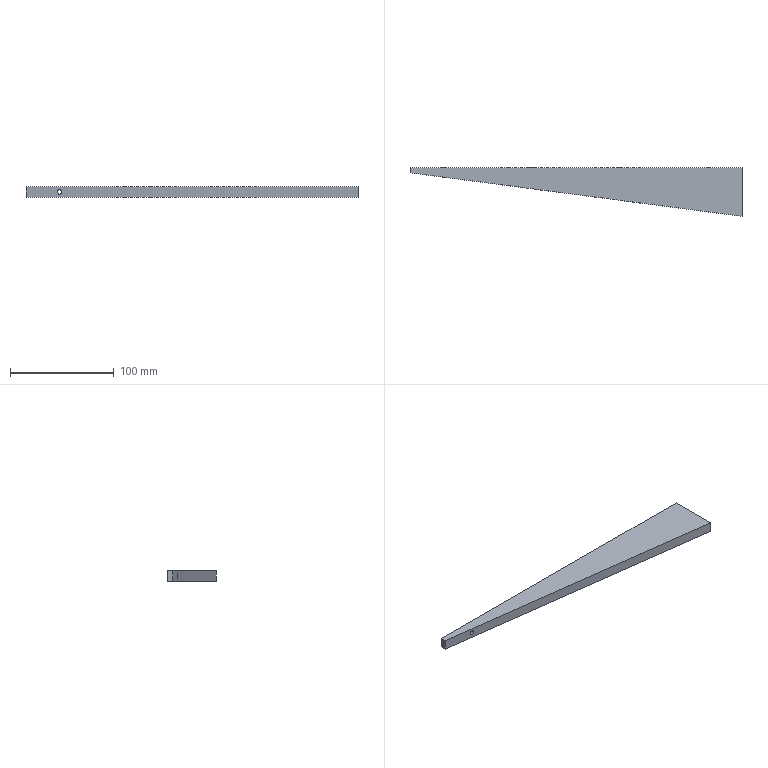Part | SolidWorks | features HoleWzd 2, Extrusion 1 | 1 solid | 32 faces | box 320 x 47 x 10 mm | volume 81873 mm3 | cylinder 14 | cone 12 | plane 6 | commonest cylinder face diameters 4.2 x14
STEP:
#1=CARTESIAN_POINT('',(-14.,41.,7.1));
#2=VERTEX_POINT('',#1);
#3=CARTESIAN_POINT('',(-14.,41.,2.9));
#4=VERTEX_POINT('',#3);
#5=CARTESIAN_POINT('',(-14.,41.,5.));
#6=DIRECTION('',(1.,0.,0.));
#7=DIRECTION('',(0.,0.,-1.));
#8=AXIS2_PLACEMENT_3D('',#5,#6,#7);
#9=CIRCLE('',#8,2.1);
#10=EDGE_CURVE('',#2,#4,#9,.T.);
#11=ORIENTED_EDGE('',*,*,#10,.F.);
#12=CARTESIAN_POINT('',(0.,41.,7.1));
#13=VERTEX_POINT('',#12);
#14=CARTESIAN_POINT('',(0.,41.,7.1));
#15=DIRECTION('',(1.,0.,0.));
#16=VECTOR('',#15,1000.);
#17=LINE('',#14,#16);
#18=EDGE_CURVE('',#2,#13,#17,.T.);
#19=ORIENTED_EDGE('',*,*,#18,.T.);
#20=CARTESIAN_POINT('',(0.,41.,2.9));
#21=VERTEX_POINT('',#20);
#22=CARTESIAN_POINT('',(0.,41.,5.));
#23=DIRECTION('',(1.,0.,0.));
#24=DIRECTION('',(0.,0.,-1.));
#25=AXIS2_PLACEMENT_3D('',#22,#23,#24);
#26=CIRCLE('',#25,2.1);
#27=EDGE_CURVE('',#13,#21,#26,.T.);
#28=ORIENTED_EDGE('',*,*,#27,.T.);
#29=CARTESIAN_POINT('',(0.,41.,2.9));
#30=DIRECTION('',(1.,0.,0.));
#31=VECTOR('',#30,1000.);
#32=LINE('',#29,#31);
#33=EDGE_CURVE('',#4,#21,#32,.T.);
#34=ORIENTED_EDGE('',*,*,#33,.F.);
#35=EDGE_LOOP('',(#11,#19,#28,#34));
#36=FACE_OUTER_BOUND('',#35,.T.);
#37=CARTESIAN_POINT('',(0.,41.,5.));
#38=DIRECTION('',(1.,0.,0.));
#39=DIRECTION('',(0.,0.,-1.));
#40=AXIS2_PLACEMENT_3D('',#37,#38,#39);
#41=CYLINDRICAL_SURFACE('',#40,2.1);
#42=ADVANCED_FACE('',(#36),#41,.F.);
#43=CARTESIAN_POINT('',(-15.262,41.,5.));
#44=VERTEX_POINT('',#43);
#45=CARTESIAN_POINT('',(-14.,41.,2.9));
#46=DIRECTION('',(0.515,0.,-0.8572));
#47=VECTOR('',#46,1000.);
#48=LINE('',#45,#47);
#49=EDGE_CURVE('',#44,#4,#48,.T.);
#50=ORIENTED_EDGE('',*,*,#49,.F.);
#51=CARTESIAN_POINT('',(-14.,41.,7.1));
#52=DIRECTION('',(0.515,0.,0.8572));
#53=VECTOR('',#52,1000.);
#54=LINE('',#51,#53);
#55=EDGE_CURVE('',#44,#2,#54,.T.);
#56=ORIENTED_EDGE('',*,*,#55,.T.);
#57=ORIENTED_EDGE('',*,*,#10,.T.);
#58=EDGE_LOOP('',(#50,#56,#57));
#59=FACE_OUTER_BOUND('',#58,.T.);
#60=CARTESIAN_POINT('',(-14.,41.,5.));
#61=DIRECTION('',(1.,0.,0.));
#62=DIRECTION('',(0.,0.,-1.));
#63=AXIS2_PLACEMENT_3D('',#60,#61,#62);
#64=CONICAL_SURFACE('',#63,2.1,1.03);
#65=ADVANCED_FACE('',(#59),#64,.F.);
#66=CARTESIAN_POINT('',(-14.,25.,7.1));
#67=VERTEX_POINT('',#66);
#68=CARTESIAN_POINT('',(-14.,25.,2.9));
#69=VERTEX_POINT('',#68);
#70=CARTESIAN_POINT('',(-14.,25.,5.));
#71=DIRECTION('',(1.,0.,0.));
#72=DIRECTION('',(0.,0.,-1.));
#73=AXIS2_PLACEMENT_3D('',#70,#71,#72);
#74=CIRCLE('',#73,2.1);
#75=EDGE_CURVE('',#67,#69,#74,.T.);
#76=ORIENTED_EDGE('',*,*,#75,.F.);
#77=CARTESIAN_POINT('',(0.,25.,7.1));
#78=VERTEX_POINT('',#77);
#79=CARTESIAN_POINT('',(0.,25.,7.1));
#80=DIRECTION('',(1.,0.,0.));
#81=VECTOR('',#80,1000.);
#82=LINE('',#79,#81);
#83=EDGE_CURVE('',#67,#78,#82,.T.);
#84=ORIENTED_EDGE('',*,*,#83,.T.);
#85=CARTESIAN_POINT('',(0.,25.,2.9));
#86=VERTEX_POINT('',#85);
#87=CARTESIAN_POINT('',(0.,25.,5.));
#88=DIRECTION('',(1.,0.,0.));
#89=DIRECTION('',(0.,0.,-1.));
#90=AXIS2_PLACEMENT_3D('',#87,#88,#89);
#91=CIRCLE('',#90,2.1);
#92=EDGE_CURVE('',#78,#86,#91,.T.);
#93=ORIENTED_EDGE('',*,*,#92,.T.);
#94=CARTESIAN_POINT('',(0.,25.,2.9));
#95=DIRECTION('',(1.,0.,0.));
#96=VECTOR('',#95,1000.);
#97=LINE('',#94,#96);
#98=EDGE_CURVE('',#69,#86,#97,.T.);
#99=ORIENTED_EDGE('',*,*,#98,.F.);
#100=EDGE_LOOP('',(#76,#84,#93,#99));
#101=FACE_OUTER_BOUND('',#100,.T.);
#102=CARTESIAN_POINT('',(0.,25.,5.));
#103=DIRECTION('',(1.,0.,0.));
#104=DIRECTION('',(0.,0.,-1.));
#105=AXIS2_PLACEMENT_3D('',#102,#103,#104);
#106=CYLINDRICAL_SURFACE('',#105,2.1);
#107=ADVANCED_FACE('',(#101),#106,.F.);
#108=CARTESIAN_POINT('',(-15.262,25.,5.));
#109=VERTEX_POINT('',#108);
#110=CARTESIAN_POINT('',(-14.,25.,2.9));
#111=DIRECTION('',(0.515,0.,-0.8572));
#112=VECTOR('',#111,1000.);
#113=LINE('',#110,#112);
#114=EDGE_CURVE('',#109,#69,#113,.T.);
#115=ORIENTED_EDGE('',*,*,#114,.F.);
#116=CARTESIAN_POINT('',(-14.,25.,7.1));
#117=DIRECTION('',(0.515,0.,0.8572));
#118=VECTOR('',#117,1000.);
#119=LINE('',#116,#118);
#120=EDGE_CURVE('',#109,#67,#119,.T.);
#121=ORIENTED_EDGE('',*,*,#120,.T.);
#122=ORIENTED_EDGE('',*,*,#75,.T.);
#123=EDGE_LOOP('',(#115,#121,#122));
#124=FACE_OUTER_BOUND('',#123,.T.);
#125=CARTESIAN_POINT('',(-14.,25.,5.));
#126=DIRECTION('',(1.,0.,0.));
#127=DIRECTION('',(0.,0.,-1.));
#128=AXIS2_PLACEMENT_3D('',#125,#126,#127);
#129=CONICAL_SURFACE('',#128,2.1,1.03);
#130=ADVANCED_FACE('',(#124),#129,.F.);
#131=CARTESIAN_POINT('',(-14.,9.,7.1));
#132=VERTEX_POINT('',#131);
#133=CARTESIAN_POINT('',(-14.,9.,2.9));
#134=VERTEX_POINT('',#133);
#135=CARTESIAN_POINT('',(-14.,9.,5.));
#136=DIRECTION('',(1.,0.,0.));
#137=DIRECTION('',(0.,0.,-1.));
#138=AXIS2_PLACEMENT_3D('',#135,#136,#137);
#139=CIRCLE('',#138,2.1);
#140=EDGE_CURVE('',#132,#134,#139,.T.);
#141=ORIENTED_EDGE('',*,*,#140,.F.);
#142=CARTESIAN_POINT('',(0.,9.,7.1));
#143=VERTEX_POINT('',#142);
#144=CARTESIAN_POINT('',(0.,9.,7.1));
#145=DIRECTION('',(1.,0.,0.));
#146=VECTOR('',#145,1000.);
#147=LINE('',#144,#146);
#148=EDGE_CURVE('',#132,#143,#147,.T.);
#149=ORIENTED_EDGE('',*,*,#148,.T.);
#150=CARTESIAN_POINT('',(0.,9.,2.9));
#151=VERTEX_POINT('',#150);
#152=CARTESIAN_POINT('',(0.,9.,5.));
#153=DIRECTION('',(1.,0.,0.));
#154=DIRECTION('',(0.,0.,-1.));
#155=AXIS2_PLACEMENT_3D('',#152,#153,#154);
#156=CIRCLE('',#155,2.1);
#157=EDGE_CURVE('',#143,#151,#156,.T.);
#158=ORIENTED_EDGE('',*,*,#157,.T.);
#159=CARTESIAN_POINT('',(0.,9.,2.9));
#160=DIRECTION('',(1.,0.,0.));
#161=VECTOR('',#160,1000.);
#162=LINE('',#159,#161);
#163=EDGE_CURVE('',#134,#151,#162,.T.);
#164=ORIENTED_EDGE('',*,*,#163,.F.);
#165=EDGE_LOOP('',(#141,#149,#158,#164));
#166=FACE_OUTER_BOUND('',#165,.T.);
#167=CARTESIAN_POINT('',(0.,9.,5.));
#168=DIRECTION('',(1.,0.,0.));
#169=DIRECTION('',(0.,0.,-1.));
#170=AXIS2_PLACEMENT_3D('',#167,#168,#169);
#171=CYLINDRICAL_SURFACE('',#170,2.1);
#172=ADVANCED_FACE('',(#166),#171,.F.);
#173=CARTESIAN_POINT('',(-15.262,9.,5.));
#174=VERTEX_POINT('',#173);
#175=CARTESIAN_POINT('',(-14.,9.,2.9));
#176=DIRECTION('',(0.515,0.,-0.8572));
#177=VECTOR('',#176,1000.);
#178=LINE('',#175,#177);
#179=EDGE_CURVE('',#174,#134,#178,.T.);
#180=ORIENTED_EDGE('',*,*,#179,.F.);
#181=CARTESIAN_POINT('',(-14.,9.,7.1));
#182=DIRECTION('',(0.515,0.,0.8572));
#183=VECTOR('',#182,1000.);
#184=LINE('',#181,#183);
#185=EDGE_CURVE('',#174,#132,#184,.T.);
#186=ORIENTED_EDGE('',*,*,#185,.T.);
#187=ORIENTED_EDGE('',*,*,#140,.T.);
#188=EDGE_LOOP('',(#180,#186,#187));
#189=FACE_OUTER_BOUND('',#188,.T.);
#190=CARTESIAN_POINT('',(-14.,9.,5.));
#191=DIRECTION('',(1.,0.,0.));
#192=DIRECTION('',(0.,0.,-1.));
#193=AXIS2_PLACEMENT_3D('',#190,#191,#192);
#194=CONICAL_SURFACE('',#193,2.1,1.03);
#195=ADVANCED_FACE('',(#189),#194,.F.);
#196=CARTESIAN_POINT('',(-287.5,37.734,2.9));
#197=VERTEX_POINT('',#196);
#198=CARTESIAN_POINT('',(-287.5,37.734,7.1));
#199=VERTEX_POINT('',#198);
#200=CARTESIAN_POINT('',(-287.5,37.734,2.9));
#201=CARTESIAN_POINT('',(-291.7,38.286,2.9));
#202=CARTESIAN_POINT('',(-291.7,38.286,7.1));
#203=CARTESIAN_POINT('',(-287.5,37.734,7.1));
#204=(BOUNDED_CURVE()B_SPLINE_CURVE(3,(#200,#201,#202,#203),.UNSPECIFIED.,.F.,.F.)B_SPLINE_CURVE_WITH_KNOTS((4,4),(4.712,7.854),.UNSPECIFIED.)CURVE()GEOMETRIC_REPRESENTATION_ITEM()RATIONAL_B_SPLINE_CURVE((1.,0.3333,0.3333,1.))REPRESENTATION_ITEM(''));
#205=EDGE_CURVE('',#197,#199,#204,.T.);
#206=ORIENTED_EDGE('',*,*,#205,.F.);
#207=CARTESIAN_POINT('',(-287.5,47.,2.9));
#208=VERTEX_POINT('',#207);
#209=CARTESIAN_POINT('',(-287.5,47.,2.9));
#210=DIRECTION('',(0.,1.,0.));
#211=VECTOR('',#210,1000.);
#212=LINE('',#209,#211);
#213=EDGE_CURVE('',#197,#208,#212,.T.);
#214=ORIENTED_EDGE('',*,*,#213,.T.);
#215=CARTESIAN_POINT('',(-287.5,47.,7.1));
#216=VERTEX_POINT('',#215);
#217=CARTESIAN_POINT('',(-287.5,47.,5.));
#218=DIRECTION('',(0.,1.,0.));
#219=DIRECTION('',(0.,0.,1.));
#220=AXIS2_PLACEMENT_3D('',#217,#218,#219);
#221=CIRCLE('',#220,2.1);
#222=EDGE_CURVE('',#208,#216,#221,.T.);
#223=ORIENTED_EDGE('',*,*,#222,.T.);
#224=CARTESIAN_POINT('',(-287.5,47.,7.1));
#225=DIRECTION('',(0.,1.,0.));
#226=VECTOR('',#225,1000.);
#227=LINE('',#224,#226);
#228=EDGE_CURVE('',#199,#216,#227,.T.);
#229=ORIENTED_EDGE('',*,*,#228,.F.);
#230=EDGE_LOOP('',(#206,#214,#223,#229));
#231=FACE_OUTER_BOUND('',#230,.T.);
#232=CARTESIAN_POINT('',(-287.5,47.,5.));
#233=DIRECTION('',(0.,1.,0.));
#234=DIRECTION('',(0.,0.,1.));
#235=AXIS2_PLACEMENT_3D('',#232,#233,#234);
#236=CYLINDRICAL_SURFACE('',#235,2.1);
#237=ADVANCED_FACE('',(#231),#236,.F.);
#238=CARTESIAN_POINT('',(-202.5,33.,2.9));
#239=VERTEX_POINT('',#238);
#240=CARTESIAN_POINT('',(-202.5,33.,7.1));
#241=VERTEX_POINT('',#240);
#242=CARTESIAN_POINT('',(-202.5,33.,5.));
#243=DIRECTION('',(0.,1.,0.));
#244=DIRECTION('',(0.,0.,1.));
#245=AXIS2_PLACEMENT_3D('',#242,#243,#244);
#246=CIRCLE('',#245,2.1);
#247=EDGE_CURVE('',#239,#241,#246,.T.);
#248=ORIENTED_EDGE('',*,*,#247,.F.);
#249=CARTESIAN_POINT('',(-202.5,47.,2.9));
#250=VERTEX_POINT('',#249);
#251=CARTESIAN_POINT('',(-202.5,47.,2.9));
#252=DIRECTION('',(0.,1.,0.));
#253=VECTOR('',#252,1000.);
#254=LINE('',#251,#253);
#255=EDGE_CURVE('',#239,#250,#254,.T.);
#256=ORIENTED_EDGE('',*,*,#255,.T.);
#257=CARTESIAN_POINT('',(-202.5,47.,7.1));
#258=VERTEX_POINT('',#257);
#259=CARTESIAN_POINT('',(-202.5,47.,5.));
#260=DIRECTION('',(0.,1.,0.));
#261=DIRECTION('',(0.,0.,1.));
#262=AXIS2_PLACEMENT_3D('',#259,#260,#261);
#263=CIRCLE('',#262,2.1);
#264=EDGE_CURVE('',#250,#258,#263,.T.);
#265=ORIENTED_EDGE('',*,*,#264,.T.);
#266=CARTESIAN_POINT('',(-202.5,47.,7.1));
#267=DIRECTION('',(0.,1.,0.));
#268=VECTOR('',#267,1000.);
#269=LINE('',#266,#268);
#270=EDGE_CURVE('',#241,#258,#269,.T.);
#271=ORIENTED_EDGE('',*,*,#270,.F.);
#272=EDGE_LOOP('',(#248,#256,#265,#271));
#273=FACE_OUTER_BOUND('',#272,.T.);
#274=CARTESIAN_POINT('',(-202.5,47.,5.));
#275=DIRECTION('',(0.,1.,0.));
#276=DIRECTION('',(0.,0.,1.));
#277=AXIS2_PLACEMENT_3D('',#274,#275,#276);
#278=CYLINDRICAL_SURFACE('',#277,2.1);
#279=ADVANCED_FACE('',(#273),#278,.F.);
#280=CARTESIAN_POINT('',(-202.5,31.738,5.));
#281=VERTEX_POINT('',#280);
#282=CARTESIAN_POINT('',(-202.5,33.,7.1));
#283=DIRECTION('',(0.,0.515,0.8572));
#284=VECTOR('',#283,1000.);
#285=LINE('',#282,#284);
#286=EDGE_CURVE('',#281,#241,#285,.T.);
#287=ORIENTED_EDGE('',*,*,#286,.F.);
#288=CARTESIAN_POINT('',(-202.5,33.,2.9));
#289=DIRECTION('',(0.,0.515,-0.8572));
#290=VECTOR('',#289,1000.);
#291=LINE('',#288,#290);
#292=EDGE_CURVE('',#281,#239,#291,.T.);
#293=ORIENTED_EDGE('',*,*,#292,.T.);
#294=ORIENTED_EDGE('',*,*,#247,.T.);
#295=EDGE_LOOP('',(#287,#293,#294));
#296=FACE_OUTER_BOUND('',#295,.T.);
#297=CARTESIAN_POINT('',(-202.5,33.,5.));
#298=DIRECTION('',(0.,1.,0.));
#299=DIRECTION('',(0.,0.,1.));
#300=AXIS2_PLACEMENT_3D('',#297,#298,#299);
#301=CONICAL_SURFACE('',#300,2.1,1.03);
#302=ADVANCED_FACE('',(#296),#301,.F.);
#303=CARTESIAN_POINT('',(-117.5,33.,2.9));
#304=VERTEX_POINT('',#303);
#305=CARTESIAN_POINT('',(-117.5,33.,7.1));
#306=VERTEX_POINT('',#305);
#307=CARTESIAN_POINT('',(-117.5,33.,5.));
#308=DIRECTION('',(0.,1.,0.));
#309=DIRECTION('',(0.,0.,1.));
#310=AXIS2_PLACEMENT_3D('',#307,#308,#309);
#311=CIRCLE('',#310,2.1);
#312=EDGE_CURVE('',#304,#306,#311,.T.);
#313=ORIENTED_EDGE('',*,*,#312,.F.);
#314=CARTESIAN_POINT('',(-117.5,47.,2.9));
#315=VERTEX_POINT('',#314);
#316=CARTESIAN_POINT('',(-117.5,47.,2.9));
#317=DIRECTION('',(0.,1.,0.));
#318=VECTOR('',#317,1000.);
#319=LINE('',#316,#318);
#320=EDGE_CURVE('',#304,#315,#319,.T.);
#321=ORIENTED_EDGE('',*,*,#320,.T.);
#322=CARTESIAN_POINT('',(-117.5,47.,7.1));
#323=VERTEX_POINT('',#322);
#324=CARTESIAN_POINT('',(-117.5,47.,5.));
#325=DIRECTION('',(0.,1.,0.));
#326=DIRECTION('',(0.,0.,1.));
#327=AXIS2_PLACEMENT_3D('',#324,#325,#326);
#328=CIRCLE('',#327,2.1);
#329=EDGE_CURVE('',#315,#323,#328,.T.);
#330=ORIENTED_EDGE('',*,*,#329,.T.);
#331=CARTESIAN_POINT('',(-117.5,47.,7.1));
#332=DIRECTION('',(0.,1.,0.));
#333=VECTOR('',#332,1000.);
#334=LINE('',#331,#333);
#335=EDGE_CURVE('',#306,#323,#334,.T.);
#336=ORIENTED_EDGE('',*,*,#335,.F.);
#337=EDGE_LOOP('',(#313,#321,#330,#336));
#338=FACE_OUTER_BOUND('',#337,.T.);
#339=CARTESIAN_POINT('',(-117.5,47.,5.));
#340=DIRECTION('',(0.,1.,0.));
#341=DIRECTION('',(0.,0.,1.));
#342=AXIS2_PLACEMENT_3D('',#339,#340,#341);
#343=CYLINDRICAL_SURFACE('',#342,2.1);
#344=ADVANCED_FACE('',(#338),#343,.F.);
#345=CARTESIAN_POINT('',(-117.5,31.738,5.));
#346=VERTEX_POINT('',#345);
#347=CARTESIAN_POINT('',(-117.5,33.,7.1));
#348=DIRECTION('',(0.,0.515,0.8572));
#349=VECTOR('',#348,1000.);
#350=LINE('',#347,#349);
#351=EDGE_CURVE('',#346,#306,#350,.T.);
#352=ORIENTED_EDGE('',*,*,#351,.F.);
#353=CARTESIAN_POINT('',(-117.5,33.,2.9));
#354=DIRECTION('',(0.,0.515,-0.8572));
#355=VECTOR('',#354,1000.);
#356=LINE('',#353,#355);
#357=EDGE_CURVE('',#346,#304,#356,.T.);
#358=ORIENTED_EDGE('',*,*,#357,.T.);
#359=ORIENTED_EDGE('',*,*,#312,.T.);
#360=EDGE_LOOP('',(#352,#358,#359));
#361=FACE_OUTER_BOUND('',#360,.T.);
#362=CARTESIAN_POINT('',(-117.5,33.,5.));
#363=DIRECTION('',(0.,1.,0.));
#364=DIRECTION('',(0.,0.,1.));
#365=AXIS2_PLACEMENT_3D('',#362,#363,#364);
#366=CONICAL_SURFACE('',#365,2.1,1.03);
#367=ADVANCED_FACE('',(#361),#366,.F.);
#368=CARTESIAN_POINT('',(-32.5,33.,2.9));
#369=VERTEX_POINT('',#368);
#370=CARTESIAN_POINT('',(-32.5,33.,7.1));
#371=VERTEX_POINT('',#370);
#372=CARTESIAN_POINT('',(-32.5,33.,5.));
#373=DIRECTION('',(0.,1.,0.));
#374=DIRECTION('',(0.,0.,1.));
#375=AXIS2_PLACEMENT_3D('',#372,#373,#374);
#376=CIRCLE('',#375,2.1);
#377=EDGE_CURVE('',#369,#371,#376,.T.);
#378=ORIENTED_EDGE('',*,*,#377,.F.);
#379=CARTESIAN_POINT('',(-32.5,47.,2.9));
#380=VERTEX_POINT('',#379);
#381=CARTESIAN_POINT('',(-32.5,47.,2.9));
#382=DIRECTION('',(0.,1.,0.));
#383=VECTOR('',#382,1000.);
#384=LINE('',#381,#383);
#385=EDGE_CURVE('',#369,#380,#384,.T.);
#386=ORIENTED_EDGE('',*,*,#385,.T.);
#387=CARTESIAN_POINT('',(-32.5,47.,7.1));
#388=VERTEX_POINT('',#387);
#389=CARTESIAN_POINT('',(-32.5,47.,5.));
#390=DIRECTION('',(0.,1.,0.));
#391=DIRECTION('',(0.,0.,1.));
#392=AXIS2_PLACEMENT_3D('',#389,#390,#391);
#393=CIRCLE('',#392,2.1);
#394=EDGE_CURVE('',#380,#388,#393,.T.);
#395=ORIENTED_EDGE('',*,*,#394,.T.);
#396=CARTESIAN_POINT('',(-32.5,47.,7.1));
#397=DIRECTION('',(0.,1.,0.));
#398=VECTOR('',#397,1000.);
#399=LINE('',#396,#398);
#400=EDGE_CURVE('',#371,#388,#399,.T.);
#401=ORIENTED_EDGE('',*,*,#400,.F.);
#402=EDGE_LOOP('',(#378,#386,#395,#401));
#403=FACE_OUTER_BOUND('',#402,.T.);
#404=CARTESIAN_POINT('',(-32.5,47.,5.));
#405=DIRECTION('',(0.,1.,0.));
#406=DIRECTION('',(0.,0.,1.));
#407=AXIS2_PLACEMENT_3D('',#404,#405,#406);
#408=CYLINDRICAL_SURFACE('',#407,2.1);
#409=ADVANCED_FACE('',(#403),#408,.F.);
#410=CARTESIAN_POINT('',(-32.5,31.738,5.));
#411=VERTEX_POINT('',#410);
#412=CARTESIAN_POINT('',(-32.5,33.,7.1));
#413=DIRECTION('',(0.,0.515,0.8572));
#414=VECTOR('',#413,1000.);
#415=LINE('',#412,#414);
#416=EDGE_CURVE('',#411,#371,#415,.T.);
#417=ORIENTED_EDGE('',*,*,#416,.F.);
#418=CARTESIAN_POINT('',(-32.5,33.,2.9));
#419=DIRECTION('',(0.,0.515,-0.8572));
#420=VECTOR('',#419,1000.);
#421=LINE('',#418,#420);
#422=EDGE_CURVE('',#411,#369,#421,.T.);
#423=ORIENTED_EDGE('',*,*,#422,.T.);
#424=ORIENTED_EDGE('',*,*,#377,.T.);
#425=EDGE_LOOP('',(#417,#423,#424));
#426=FACE_OUTER_BOUND('',#425,.T.);
#427=CARTESIAN_POINT('',(-32.5,33.,5.));
#428=DIRECTION('',(0.,1.,0.));
#429=DIRECTION('',(0.,0.,1.));
#430=AXIS2_PLACEMENT_3D('',#427,#428,#429);
#431=CONICAL_SURFACE('',#430,2.1,1.03);
#432=ADVANCED_FACE('',(#426),#431,.F.);
#433=CARTESIAN_POINT('',(0.,41.,5.));
#434=DIRECTION('',(1.,0.,0.));
#435=DIRECTION('',(0.,0.,-1.));
#436=AXIS2_PLACEMENT_3D('',#433,#434,#435);
#437=CIRCLE('',#436,2.1);
#438=EDGE_CURVE('',#21,#13,#437,.T.);
#439=ORIENTED_EDGE('',*,*,#438,.F.);
#440=ORIENTED_EDGE('',*,*,#27,.F.);
#441=EDGE_LOOP('',(#439,#440));
#442=FACE_BOUND('',#441,.T.);
#443=CARTESIAN_POINT('',(0.,25.,5.));
#444=DIRECTION('',(1.,0.,0.));
#445=DIRECTION('',(0.,0.,-1.));
#446=AXIS2_PLACEMENT_3D('',#443,#444,#445);
#447=CIRCLE('',#446,2.1);
#448=EDGE_CURVE('',#86,#78,#447,.T.);
#449=ORIENTED_EDGE('',*,*,#448,.F.);
#450=ORIENTED_EDGE('',*,*,#92,.F.);
#451=EDGE_LOOP('',(#449,#450));
#452=FACE_BOUND('',#451,.T.);
#453=CARTESIAN_POINT('',(0.,9.,5.));
#454=DIRECTION('',(1.,0.,0.));
#455=DIRECTION('',(0.,0.,-1.));
#456=AXIS2_PLACEMENT_3D('',#453,#454,#455);
#457=CIRCLE('',#456,2.1);
#458=EDGE_CURVE('',#151,#143,#457,.T.);
#459=ORIENTED_EDGE('',*,*,#458,.F.);
#460=ORIENTED_EDGE('',*,*,#157,.F.);
#461=EDGE_LOOP('',(#459,#460));
#462=FACE_BOUND('',#461,.T.);
#463=CARTESIAN_POINT('',(0.,0.,0.));
#464=VERTEX_POINT('',#463);
#465=CARTESIAN_POINT('',(0.,47.,0.));
#466=VERTEX_POINT('',#465);
#467=CARTESIAN_POINT('',(0.,47.,0.));
#468=DIRECTION('',(0.,1.,0.));
#469=VECTOR('',#468,1000.);
#470=LINE('',#467,#469);
#471=EDGE_CURVE('',#464,#466,#470,.T.);
#472=ORIENTED_EDGE('',*,*,#471,.T.);
#473=CARTESIAN_POINT('',(0.,47.,10.));
#474=VERTEX_POINT('',#473);
#475=CARTESIAN_POINT('',(0.,47.,10.));
#476=DIRECTION('',(0.,0.,-1.));
#477=VECTOR('',#476,1000.);
#478=LINE('',#475,#477);
#479=EDGE_CURVE('',#474,#466,#478,.T.);
#480=ORIENTED_EDGE('',*,*,#479,.F.);
#481=CARTESIAN_POINT('',(0.,0.,10.));
#482=VERTEX_POINT('',#481);
#483=CARTESIAN_POINT('',(0.,47.,10.));
#484=DIRECTION('',(0.,1.,0.));
#485=VECTOR('',#484,1000.);
#486=LINE('',#483,#485);
#487=EDGE_CURVE('',#482,#474,#486,.T.);
#488=ORIENTED_EDGE('',*,*,#487,.F.);
#489=CARTESIAN_POINT('',(0.,0.,10.));
#490=DIRECTION('',(0.,0.,-1.));
#491=VECTOR('',#490,1000.);
#492=LINE('',#489,#491);
#493=EDGE_CURVE('',#482,#464,#492,.T.);
#494=ORIENTED_EDGE('',*,*,#493,.T.);
#495=EDGE_LOOP('',(#472,#480,#488,#494));
#496=FACE_OUTER_BOUND('',#495,.T.);
#497=CARTESIAN_POINT('',(0.,47.,10.));
#498=DIRECTION('',(-1.,0.,0.));
#499=DIRECTION('',(0.,-1.,0.));
#500=AXIS2_PLACEMENT_3D('',#497,#498,#499);
#501=PLANE('',#500);
#502=ADVANCED_FACE('',(#442,#452,#462,#496),#501,.F.);
#503=CARTESIAN_POINT('',(-287.5,47.,5.));
#504=DIRECTION('',(0.,1.,0.));
#505=DIRECTION('',(0.,0.,1.));
#506=AXIS2_PLACEMENT_3D('',#503,#504,#505);
#507=CIRCLE('',#506,2.1);
#508=EDGE_CURVE('',#216,#208,#507,.T.);
#509=ORIENTED_EDGE('',*,*,#508,.F.);
#510=ORIENTED_EDGE('',*,*,#222,.F.);
#511=EDGE_LOOP('',(#509,#510));
#512=FACE_BOUND('',#511,.T.);
#513=CARTESIAN_POINT('',(-202.5,47.,5.));
#514=DIRECTION('',(0.,1.,0.));
#515=DIRECTION('',(0.,0.,1.));
#516=AXIS2_PLACEMENT_3D('',#513,#514,#515);
#517=CIRCLE('',#516,2.1);
#518=EDGE_CURVE('',#258,#250,#517,.T.);
#519=ORIENTED_EDGE('',*,*,#518,.F.);
#520=ORIENTED_EDGE('',*,*,#264,.F.);
#521=EDGE_LOOP('',(#519,#520));
#522=FACE_BOUND('',#521,.T.);
#523=CARTESIAN_POINT('',(-117.5,47.,5.));
#524=DIRECTION('',(0.,1.,0.));
#525=DIRECTION('',(0.,0.,1.));
#526=AXIS2_PLACEMENT_3D('',#523,#524,#525);
#527=CIRCLE('',#526,2.1);
#528=EDGE_CURVE('',#323,#315,#527,.T.);
#529=ORIENTED_EDGE('',*,*,#528,.F.);
#530=ORIENTED_EDGE('',*,*,#329,.F.);
#531=EDGE_LOOP('',(#529,#530));
#532=FACE_BOUND('',#531,.T.);
#533=CARTESIAN_POINT('',(-32.5,47.,5.));
#534=DIRECTION('',(0.,1.,0.));
#535=DIRECTION('',(0.,0.,1.));
#536=AXIS2_PLACEMENT_3D('',#533,#534,#535);
#537=CIRCLE('',#536,2.1);
#538=EDGE_CURVE('',#388,#380,#537,.T.);
#539=ORIENTED_EDGE('',*,*,#538,.F.);
#540=ORIENTED_EDGE('',*,*,#394,.F.);
#541=EDGE_LOOP('',(#539,#540));
#542=FACE_BOUND('',#541,.T.);
#543=CARTESIAN_POINT('',(-320.,47.,0.));
#544=VERTEX_POINT('',#543);
#545=CARTESIAN_POINT('',(-320.,47.,0.));
#546=DIRECTION('',(-1.,0.,0.));
#547=VECTOR('',#546,1000.);
#548=LINE('',#545,#547);
#549=EDGE_CURVE('',#466,#544,#548,.T.);
#550=ORIENTED_EDGE('',*,*,#549,.T.);
#551=CARTESIAN_POINT('',(-320.,47.,10.));
#552=VERTEX_POINT('',#551);
#553=CARTESIAN_POINT('',(-320.,47.,10.));
#554=DIRECTION('',(0.,0.,-1.));
#555=VECTOR('',#554,1000.);
#556=LINE('',#553,#555);
#557=EDGE_CURVE('',#552,#544,#556,.T.);
#558=ORIENTED_EDGE('',*,*,#557,.F.);
#559=CARTESIAN_POINT('',(-320.,47.,10.));
#560=DIRECTION('',(-1.,0.,0.));
#561=VECTOR('',#560,1000.);
#562=LINE('',#559,#561);
#563=EDGE_CURVE('',#474,#552,#562,.T.);
#564=ORIENTED_EDGE('',*,*,#563,.F.);
#565=ORIENTED_EDGE('',*,*,#479,.T.);
#566=EDGE_LOOP('',(#550,#558,#564,#565));
#567=FACE_OUTER_BOUND('',#566,.T.);
#568=CARTESIAN_POINT('',(-320.,47.,10.));
#569=DIRECTION('',(0.,-1.,0.));
#570=DIRECTION('',(0.,0.,-1.));
#571=AXIS2_PLACEMENT_3D('',#568,#569,#570);
#572=PLANE('',#571);
#573=ADVANCED_FACE('',(#512,#522,#532,#542,#567),#572,.F.);
#574=CARTESIAN_POINT('',(-320.,42.,0.));
#575=VERTEX_POINT('',#574);
#576=CARTESIAN_POINT('',(-320.,47.,0.));
#577=DIRECTION('',(0.,-1.,0.));
#578=VECTOR('',#577,1000.);
#579=LINE('',#576,#578);
#580=EDGE_CURVE('',#544,#575,#579,.T.);
#581=ORIENTED_EDGE('',*,*,#580,.T.);
#582=CARTESIAN_POINT('',(-320.,42.,10.));
#583=VERTEX_POINT('',#582);
#584=CARTESIAN_POINT('',(-320.,42.,10.));
#585=DIRECTION('',(0.,0.,-1.));
#586=VECTOR('',#585,1000.);
#587=LINE('',#584,#586);
#588=EDGE_CURVE('',#583,#575,#587,.T.);
#589=ORIENTED_EDGE('',*,*,#588,.F.);
#590=CARTESIAN_POINT('',(-320.,47.,10.));
#591=DIRECTION('',(0.,-1.,0.));
#592=VECTOR('',#591,1000.);
#593=LINE('',#590,#592);
#594=EDGE_CURVE('',#552,#583,#593,.T.);
#595=ORIENTED_EDGE('',*,*,#594,.F.);
#596=ORIENTED_EDGE('',*,*,#557,.T.);
#597=EDGE_LOOP('',(#581,#589,#595,#596));
#598=FACE_OUTER_BOUND('',#597,.T.);
#599=CARTESIAN_POINT('',(-320.,47.,10.));
#600=DIRECTION('',(1.,0.,0.));
#601=DIRECTION('',(0.,0.,-1.));
#602=AXIS2_PLACEMENT_3D('',#599,#600,#601);
#603=PLANE('',#602);
#604=ADVANCED_FACE('',(#598),#603,.F.);
#605=CARTESIAN_POINT('',(-287.5,37.734,7.1));
#606=CARTESIAN_POINT('',(-283.3,37.183,7.1));
#607=CARTESIAN_POINT('',(-283.3,37.183,2.9));
#608=CARTESIAN_POINT('',(-287.5,37.734,2.9));
#609=(BOUNDED_CURVE()B_SPLINE_CURVE(3,(#605,#606,#607,#608),.UNSPECIFIED.,.F.,.F.)B_SPLINE_CURVE_WITH_KNOTS((4,4),(1.571,4.712),.UNSPECIFIED.)CURVE()GEOMETRIC_REPRESENTATION_ITEM()RATIONAL_B_SPLINE_CURVE((1.,0.3333,0.3333,1.))REPRESENTATION_ITEM(''));
#610=EDGE_CURVE('',#199,#197,#609,.T.);
#611=ORIENTED_EDGE('',*,*,#610,.T.);
#612=ORIENTED_EDGE('',*,*,#205,.T.);
#613=EDGE_LOOP('',(#611,#612));
#614=FACE_BOUND('',#613,.T.);
#615=CARTESIAN_POINT('',(0.,0.,0.));
#616=DIRECTION('',(0.9915,-0.1301,0.));
#617=VECTOR('',#616,1000.);
#618=LINE('',#615,#617);
#619=EDGE_CURVE('',#575,#464,#618,.T.);
#620=ORIENTED_EDGE('',*,*,#619,.T.);
#621=ORIENTED_EDGE('',*,*,#493,.F.);
#622=CARTESIAN_POINT('',(0.,0.,10.));
#623=DIRECTION('',(0.9915,-0.1301,0.));
#624=VECTOR('',#623,1000.);
#625=LINE('',#622,#624);
#626=EDGE_CURVE('',#583,#482,#625,.T.);
#627=ORIENTED_EDGE('',*,*,#626,.F.);
#628=ORIENTED_EDGE('',*,*,#588,.T.);
#629=EDGE_LOOP('',(#620,#621,#627,#628));
#630=FACE_OUTER_BOUND('',#629,.T.);
#631=CARTESIAN_POINT('',(0.,0.,10.));
#632=DIRECTION('',(0.1301,0.9915,0.));
#633=DIRECTION('',(-0.9915,0.1301,0.));
#634=AXIS2_PLACEMENT_3D('',#631,#632,#633);
#635=PLANE('',#634);
#636=ADVANCED_FACE('',(#614,#630),#635,.F.);
#637=ORIENTED_EDGE('',*,*,#487,.T.);
#638=ORIENTED_EDGE('',*,*,#563,.T.);
#639=ORIENTED_EDGE('',*,*,#594,.T.);
#640=ORIENTED_EDGE('',*,*,#626,.T.);
#641=EDGE_LOOP('',(#637,#638,#639,#640));
#642=FACE_OUTER_BOUND('',#641,.T.);
#643=CARTESIAN_POINT('',(0.,0.,10.));
#644=DIRECTION('',(0.,0.,1.));
#645=DIRECTION('',(1.,0.,0.));
#646=AXIS2_PLACEMENT_3D('',#643,#644,#645);
#647=PLANE('',#646);
#648=ADVANCED_FACE('',(#642),#647,.T.);
#649=ORIENTED_EDGE('',*,*,#471,.F.);
#650=ORIENTED_EDGE('',*,*,#619,.F.);
#651=ORIENTED_EDGE('',*,*,#580,.F.);
#652=ORIENTED_EDGE('',*,*,#549,.F.);
#653=EDGE_LOOP('',(#649,#650,#651,#652));
#654=FACE_OUTER_BOUND('',#653,.T.);
#655=CARTESIAN_POINT('',(0.,0.,0.));
#656=DIRECTION('',(0.,0.,1.));
#657=DIRECTION('',(1.,0.,0.));
#658=AXIS2_PLACEMENT_3D('',#655,#656,#657);
#659=PLANE('',#658);
#660=ADVANCED_FACE('',(#654),#659,.F.);
#661=ORIENTED_EDGE('',*,*,#422,.F.);
#662=ORIENTED_EDGE('',*,*,#416,.T.);
#663=CARTESIAN_POINT('',(-32.5,33.,5.));
#664=DIRECTION('',(0.,1.,0.));
#665=DIRECTION('',(0.,0.,1.));
#666=AXIS2_PLACEMENT_3D('',#663,#664,#665);
#667=CIRCLE('',#666,2.1);
#668=EDGE_CURVE('',#371,#369,#667,.T.);
#669=ORIENTED_EDGE('',*,*,#668,.T.);
#670=EDGE_LOOP('',(#661,#662,#669));
#671=FACE_OUTER_BOUND('',#670,.T.);
#672=CARTESIAN_POINT('',(-32.5,33.,5.));
#673=DIRECTION('',(0.,1.,0.));
#674=DIRECTION('',(0.,0.,1.));
#675=AXIS2_PLACEMENT_3D('',#672,#673,#674);
#676=CONICAL_SURFACE('',#675,2.1,1.03);
#677=ADVANCED_FACE('',(#671),#676,.F.);
#678=ORIENTED_EDGE('',*,*,#385,.F.);
#679=ORIENTED_EDGE('',*,*,#668,.F.);
#680=ORIENTED_EDGE('',*,*,#400,.T.);
#681=ORIENTED_EDGE('',*,*,#538,.T.);
#682=EDGE_LOOP('',(#678,#679,#680,#681));
#683=FACE_OUTER_BOUND('',#682,.T.);
#684=CARTESIAN_POINT('',(-32.5,47.,5.));
#685=DIRECTION('',(0.,1.,0.));
#686=DIRECTION('',(0.,0.,1.));
#687=AXIS2_PLACEMENT_3D('',#684,#685,#686);
#688=CYLINDRICAL_SURFACE('',#687,2.1);
#689=ADVANCED_FACE('',(#683),#688,.F.);
#690=ORIENTED_EDGE('',*,*,#357,.F.);
#691=ORIENTED_EDGE('',*,*,#351,.T.);
#692=CARTESIAN_POINT('',(-117.5,33.,5.));
#693=DIRECTION('',(0.,1.,0.));
#694=DIRECTION('',(0.,0.,1.));
#695=AXIS2_PLACEMENT_3D('',#692,#693,#694);
#696=CIRCLE('',#695,2.1);
#697=EDGE_CURVE('',#306,#304,#696,.T.);
#698=ORIENTED_EDGE('',*,*,#697,.T.);
#699=EDGE_LOOP('',(#690,#691,#698));
#700=FACE_OUTER_BOUND('',#699,.T.);
#701=CARTESIAN_POINT('',(-117.5,33.,5.));
#702=DIRECTION('',(0.,1.,0.));
#703=DIRECTION('',(0.,0.,1.));
#704=AXIS2_PLACEMENT_3D('',#701,#702,#703);
#705=CONICAL_SURFACE('',#704,2.1,1.03);
#706=ADVANCED_FACE('',(#700),#705,.F.);
#707=ORIENTED_EDGE('',*,*,#320,.F.);
#708=ORIENTED_EDGE('',*,*,#697,.F.);
#709=ORIENTED_EDGE('',*,*,#335,.T.);
#710=ORIENTED_EDGE('',*,*,#528,.T.);
#711=EDGE_LOOP('',(#707,#708,#709,#710));
#712=FACE_OUTER_BOUND('',#711,.T.);
#713=CARTESIAN_POINT('',(-117.5,47.,5.));
#714=DIRECTION('',(0.,1.,0.));
#715=DIRECTION('',(0.,0.,1.));
#716=AXIS2_PLACEMENT_3D('',#713,#714,#715);
#717=CYLINDRICAL_SURFACE('',#716,2.1);
#718=ADVANCED_FACE('',(#712),#717,.F.);
#719=ORIENTED_EDGE('',*,*,#292,.F.);
#720=ORIENTED_EDGE('',*,*,#286,.T.);
#721=CARTESIAN_POINT('',(-202.5,33.,5.));
#722=DIRECTION('',(0.,1.,0.));
#723=DIRECTION('',(0.,0.,1.));
#724=AXIS2_PLACEMENT_3D('',#721,#722,#723);
#725=CIRCLE('',#724,2.1);
#726=EDGE_CURVE('',#241,#239,#725,.T.);
#727=ORIENTED_EDGE('',*,*,#726,.T.);
#728=EDGE_LOOP('',(#719,#720,#727));
#729=FACE_OUTER_BOUND('',#728,.T.);
#730=CARTESIAN_POINT('',(-202.5,33.,5.));
#731=DIRECTION('',(0.,1.,0.));
#732=DIRECTION('',(0.,0.,1.));
#733=AXIS2_PLACEMENT_3D('',#730,#731,#732);
#734=CONICAL_SURFACE('',#733,2.1,1.03);
#735=ADVANCED_FACE('',(#729),#734,.F.);
#736=ORIENTED_EDGE('',*,*,#255,.F.);
#737=ORIENTED_EDGE('',*,*,#726,.F.);
#738=ORIENTED_EDGE('',*,*,#270,.T.);
#739=ORIENTED_EDGE('',*,*,#518,.T.);
#740=EDGE_LOOP('',(#736,#737,#738,#739));
#741=FACE_OUTER_BOUND('',#740,.T.);
#742=CARTESIAN_POINT('',(-202.5,47.,5.));
#743=DIRECTION('',(0.,1.,0.));
#744=DIRECTION('',(0.,0.,1.));
#745=AXIS2_PLACEMENT_3D('',#742,#743,#744);
#746=CYLINDRICAL_SURFACE('',#745,2.1);
#747=ADVANCED_FACE('',(#741),#746,.F.);
#748=ORIENTED_EDGE('',*,*,#213,.F.);
#749=ORIENTED_EDGE('',*,*,#610,.F.);
#750=ORIENTED_EDGE('',*,*,#228,.T.);
#751=ORIENTED_EDGE('',*,*,#508,.T.);
#752=EDGE_LOOP('',(#748,#749,#750,#751));
#753=FACE_OUTER_BOUND('',#752,.T.);
#754=CARTESIAN_POINT('',(-287.5,47.,5.));
#755=DIRECTION('',(0.,1.,0.));
#756=DIRECTION('',(0.,0.,1.));
#757=AXIS2_PLACEMENT_3D('',#754,#755,#756);
#758=CYLINDRICAL_SURFACE('',#757,2.1);
#759=ADVANCED_FACE('',(#753),#758,.F.);
#760=ORIENTED_EDGE('',*,*,#185,.F.);
#761=ORIENTED_EDGE('',*,*,#179,.T.);
#762=CARTESIAN_POINT('',(-14.,9.,5.));
#763=DIRECTION('',(1.,0.,0.));
#764=DIRECTION('',(0.,0.,-1.));
#765=AXIS2_PLACEMENT_3D('',#762,#763,#764);
#766=CIRCLE('',#765,2.1);
#767=EDGE_CURVE('',#134,#132,#766,.T.);
#768=ORIENTED_EDGE('',*,*,#767,.T.);
#769=EDGE_LOOP('',(#760,#761,#768));
#770=FACE_OUTER_BOUND('',#769,.T.);
#771=CARTESIAN_POINT('',(-14.,9.,5.));
#772=DIRECTION('',(1.,0.,0.));
#773=DIRECTION('',(0.,0.,-1.));
#774=AXIS2_PLACEMENT_3D('',#771,#772,#773);
#775=CONICAL_SURFACE('',#774,2.1,1.03);
#776=ADVANCED_FACE('',(#770),#775,.F.);
#777=ORIENTED_EDGE('',*,*,#148,.F.);
#778=ORIENTED_EDGE('',*,*,#767,.F.);
#779=ORIENTED_EDGE('',*,*,#163,.T.);
#780=ORIENTED_EDGE('',*,*,#458,.T.);
#781=EDGE_LOOP('',(#777,#778,#779,#780));
#782=FACE_OUTER_BOUND('',#781,.T.);
#783=CARTESIAN_POINT('',(0.,9.,5.));
#784=DIRECTION('',(1.,0.,0.));
#785=DIRECTION('',(0.,0.,-1.));
#786=AXIS2_PLACEMENT_3D('',#783,#784,#785);
#787=CYLINDRICAL_SURFACE('',#786,2.1);
#788=ADVANCED_FACE('',(#782),#787,.F.);
#789=ORIENTED_EDGE('',*,*,#120,.F.);
#790=ORIENTED_EDGE('',*,*,#114,.T.);
#791=CARTESIAN_POINT('',(-14.,25.,5.));
#792=DIRECTION('',(1.,0.,0.));
#793=DIRECTION('',(0.,0.,-1.));
#794=AXIS2_PLACEMENT_3D('',#791,#792,#793);
#795=CIRCLE('',#794,2.1);
#796=EDGE_CURVE('',#69,#67,#795,.T.);
#797=ORIENTED_EDGE('',*,*,#796,.T.);
#798=EDGE_LOOP('',(#789,#790,#797));
#799=FACE_OUTER_BOUND('',#798,.T.);
#800=CARTESIAN_POINT('',(-14.,25.,5.));
#801=DIRECTION('',(1.,0.,0.));
#802=DIRECTION('',(0.,0.,-1.));
#803=AXIS2_PLACEMENT_3D('',#800,#801,#802);
#804=CONICAL_SURFACE('',#803,2.1,1.03);
#805=ADVANCED_FACE('',(#799),#804,.F.);
#806=ORIENTED_EDGE('',*,*,#83,.F.);
#807=ORIENTED_EDGE('',*,*,#796,.F.);
#808=ORIENTED_EDGE('',*,*,#98,.T.);
#809=ORIENTED_EDGE('',*,*,#448,.T.);
#810=EDGE_LOOP('',(#806,#807,#808,#809));
#811=FACE_OUTER_BOUND('',#810,.T.);
#812=CARTESIAN_POINT('',(0.,25.,5.));
#813=DIRECTION('',(1.,0.,0.));
#814=DIRECTION('',(0.,0.,-1.));
#815=AXIS2_PLACEMENT_3D('',#812,#813,#814);
#816=CYLINDRICAL_SURFACE('',#815,2.1);
#817=ADVANCED_FACE('',(#811),#816,.F.);
#818=ORIENTED_EDGE('',*,*,#55,.F.);
#819=ORIENTED_EDGE('',*,*,#49,.T.);
#820=CARTESIAN_POINT('',(-14.,41.,5.));
#821=DIRECTION('',(1.,0.,0.));
#822=DIRECTION('',(0.,0.,-1.));
#823=AXIS2_PLACEMENT_3D('',#820,#821,#822);
#824=CIRCLE('',#823,2.1);
#825=EDGE_CURVE('',#4,#2,#824,.T.);
#826=ORIENTED_EDGE('',*,*,#825,.T.);
#827=EDGE_LOOP('',(#818,#819,#826));
#828=FACE_OUTER_BOUND('',#827,.T.);
#829=CARTESIAN_POINT('',(-14.,41.,5.));
#830=DIRECTION('',(1.,0.,0.));
#831=DIRECTION('',(0.,0.,-1.));
#832=AXIS2_PLACEMENT_3D('',#829,#830,#831);
#833=CONICAL_SURFACE('',#832,2.1,1.03);
#834=ADVANCED_FACE('',(#828),#833,.F.);
#835=ORIENTED_EDGE('',*,*,#18,.F.);
#836=ORIENTED_EDGE('',*,*,#825,.F.);
#837=ORIENTED_EDGE('',*,*,#33,.T.);
#838=ORIENTED_EDGE('',*,*,#438,.T.);
#839=EDGE_LOOP('',(#835,#836,#837,#838));
#840=FACE_OUTER_BOUND('',#839,.T.);
#841=CARTESIAN_POINT('',(0.,41.,5.));
#842=DIRECTION('',(1.,0.,0.));
#843=DIRECTION('',(0.,0.,-1.));
#844=AXIS2_PLACEMENT_3D('',#841,#842,#843);
#845=CYLINDRICAL_SURFACE('',#844,2.1);
#846=ADVANCED_FACE('',(#840),#845,.F.);
#847=CLOSED_SHELL('',(#42,#65,#107,#130,#172,#195,#237,#279,#302,#344,#367,#409,#432,#502,#573,#604,#636,#648,#660,#677,#689,#706,#718,#735,#747,#759,#776,#788,#805,#817,#834,#846));
#848=MANIFOLD_SOLID_BREP('',#847);
#849=CARTESIAN_POINT('',(0.,0.,0.));
#850=DIRECTION('',(0.,0.,1.));
#851=DIRECTION('',(1.,0.,0.));
#852=AXIS2_PLACEMENT_3D('',#849,#850,#851);
#853=(LENGTH_UNIT()NAMED_UNIT(*)SI_UNIT(.MILLI.,.METRE.));
#854=UNCERTAINTY_MEASURE_WITH_UNIT(LENGTH_MEASURE(0.00001),#853,'','');
#855=(NAMED_UNIT(*)PLANE_ANGLE_UNIT()SI_UNIT($,.RADIAN.));
#856=(NAMED_UNIT(*)SI_UNIT($,.STERADIAN.)SOLID_ANGLE_UNIT());
#857=(GEOMETRIC_REPRESENTATION_CONTEXT(3)GLOBAL_UNCERTAINTY_ASSIGNED_CONTEXT((#854))GLOBAL_UNIT_ASSIGNED_CONTEXT((#853,#855,#856))REPRESENTATION_CONTEXT('',''));
#858=ADVANCED_BREP_SHAPE_REPRESENTATION('',(#848,#852),#857);